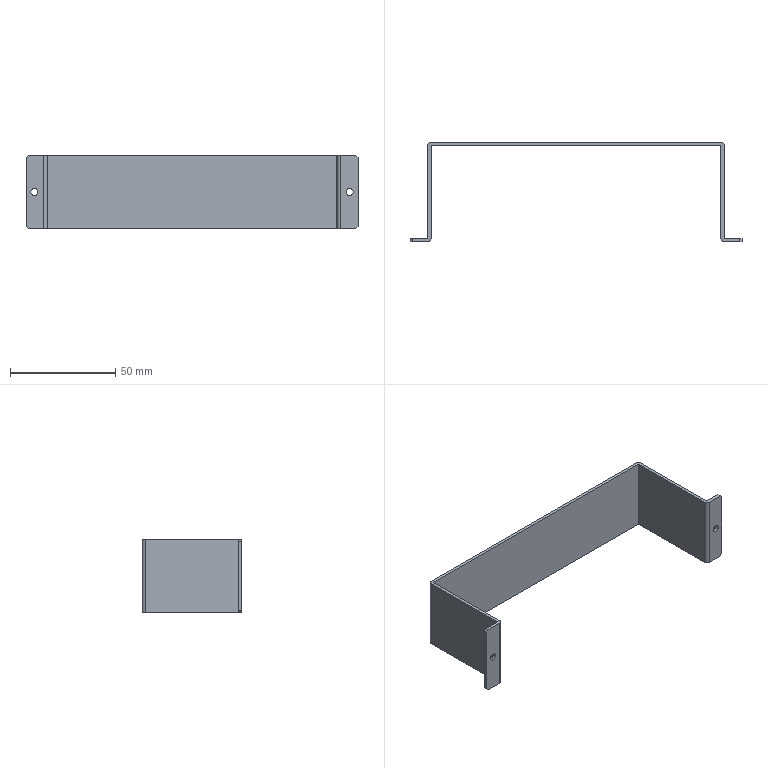Part | NX | 1 solid | 24 faces | box 158 x 47.5 x 35 mm | volume 13029 mm3 | plane 18 | cylinder 6 | commonest cylinder face diameters 3 x4 3.3 x2
STEP:
#1=CARTESIAN_POINT('',(-70.5,-1.5,35.));
#2=VERTEX_POINT('',#1);
#3=CARTESIAN_POINT('',(-70.5,-46.,35.));
#4=VERTEX_POINT('',#3);
#5=CARTESIAN_POINT('',(-70.5,0.,35.));
#6=DIRECTION('',(0.,-1.,0.));
#7=VECTOR('',#6,1000.);
#8=LINE('',#5,#7);
#9=EDGE_CURVE('',#2,#4,#8,.T.);
#10=ORIENTED_EDGE('',*,*,#9,.F.);
#11=CARTESIAN_POINT('',(-70.5,-1.5,0.));
#12=VERTEX_POINT('',#11);
#13=CARTESIAN_POINT('',(-70.5,-1.5,35.));
#14=DIRECTION('',(0.,0.,-1.));
#15=VECTOR('',#14,1000.);
#16=LINE('',#13,#15);
#17=EDGE_CURVE('',#2,#12,#16,.T.);
#18=ORIENTED_EDGE('',*,*,#17,.T.);
#19=CARTESIAN_POINT('',(-70.5,-46.,0.));
#20=VERTEX_POINT('',#19);
#21=CARTESIAN_POINT('',(-70.5,0.,0.));
#22=DIRECTION('',(0.,-1.,0.));
#23=VECTOR('',#22,1000.);
#24=LINE('',#21,#23);
#25=EDGE_CURVE('',#12,#20,#24,.T.);
#26=ORIENTED_EDGE('',*,*,#25,.T.);
#27=CARTESIAN_POINT('',(-70.5,-46.,35.));
#28=DIRECTION('',(0.,0.,-1.));
#29=VECTOR('',#28,1000.);
#30=LINE('',#27,#29);
#31=EDGE_CURVE('',#4,#20,#30,.T.);
#32=ORIENTED_EDGE('',*,*,#31,.F.);
#33=EDGE_LOOP('',(#10,#18,#26,#32));
#34=FACE_BOUND('',#33,.T.);
#35=CARTESIAN_POINT('',(-70.5,0.,35.));
#36=DIRECTION('',(1.,0.,0.));
#37=DIRECTION('',(0.,0.,-1.));
#38=AXIS2_PLACEMENT_3D('',#35,#36,#37);
#39=PLANE('',#38);
#40=ADVANCED_FACE('',(#34),#39,.F.);
#41=CARTESIAN_POINT('',(-75.,-46.,19.15));
#42=VERTEX_POINT('',#41);
#43=CARTESIAN_POINT('',(-75.,-46.,17.5));
#44=DIRECTION('',(0.,1.,0.));
#45=DIRECTION('',(0.,0.,1.));
#46=AXIS2_PLACEMENT_3D('',#43,#44,#45);
#47=CIRCLE('',#46,1.65);
#48=EDGE_CURVE('',#42,#42,#47,.T.);
#49=ORIENTED_EDGE('',*,*,#48,.F.);
#50=EDGE_LOOP('',(#49));
#51=FACE_BOUND('',#50,.T.);
#52=CARTESIAN_POINT('',(-78.,-46.,0.));
#53=VERTEX_POINT('',#52);
#54=CARTESIAN_POINT('',(-70.5,-46.,0.));
#55=DIRECTION('',(-1.,0.,0.));
#56=VECTOR('',#55,1000.);
#57=LINE('',#54,#56);
#58=EDGE_CURVE('',#20,#53,#57,.T.);
#59=ORIENTED_EDGE('',*,*,#58,.T.);
#60=CARTESIAN_POINT('',(-79.,-46.,1.));
#61=VERTEX_POINT('',#60);
#62=CARTESIAN_POINT('',(-79.,-46.,1.));
#63=DIRECTION('',(-0.7071,0.,0.7071));
#64=VECTOR('',#63,1000.);
#65=LINE('',#62,#64);
#66=EDGE_CURVE('',#53,#61,#65,.T.);
#67=ORIENTED_EDGE('',*,*,#66,.T.);
#68=CARTESIAN_POINT('',(-79.,-46.,34.));
#69=VERTEX_POINT('',#68);
#70=CARTESIAN_POINT('',(-79.,-46.,35.));
#71=DIRECTION('',(0.,0.,-1.));
#72=VECTOR('',#71,1000.);
#73=LINE('',#70,#72);
#74=EDGE_CURVE('',#69,#61,#73,.T.);
#75=ORIENTED_EDGE('',*,*,#74,.F.);
#76=CARTESIAN_POINT('',(-78.,-46.,35.));
#77=VERTEX_POINT('',#76);
#78=CARTESIAN_POINT('',(-78.,-46.,35.));
#79=DIRECTION('',(-0.7071,0.,-0.7071));
#80=VECTOR('',#79,1000.);
#81=LINE('',#78,#80);
#82=EDGE_CURVE('',#69,#77,#81,.F.);
#83=ORIENTED_EDGE('',*,*,#82,.T.);
#84=CARTESIAN_POINT('',(-70.5,-46.,35.));
#85=DIRECTION('',(-1.,0.,0.));
#86=VECTOR('',#85,1000.);
#87=LINE('',#84,#86);
#88=EDGE_CURVE('',#4,#77,#87,.T.);
#89=ORIENTED_EDGE('',*,*,#88,.F.);
#90=ORIENTED_EDGE('',*,*,#31,.T.);
#91=EDGE_LOOP('',(#59,#67,#75,#83,#89,#90));
#92=FACE_BOUND('',#91,.T.);
#93=CARTESIAN_POINT('',(-70.5,-46.,35.));
#94=DIRECTION('',(0.,-1.,0.));
#95=DIRECTION('',(0.,0.,-1.));
#96=AXIS2_PLACEMENT_3D('',#93,#94,#95);
#97=PLANE('',#96);
#98=ADVANCED_FACE('',(#51,#92),#97,.F.);
#99=ORIENTED_EDGE('',*,*,#74,.T.);
#100=CARTESIAN_POINT('',(-79.,-47.5,1.));
#101=VERTEX_POINT('',#100);
#102=CARTESIAN_POINT('',(-79.,-47.5,1.));
#103=DIRECTION('',(0.,-1.,0.));
#104=VECTOR('',#103,1000.);
#105=LINE('',#102,#104);
#106=EDGE_CURVE('',#61,#101,#105,.T.);
#107=ORIENTED_EDGE('',*,*,#106,.T.);
#108=CARTESIAN_POINT('',(-79.,-47.5,34.));
#109=VERTEX_POINT('',#108);
#110=CARTESIAN_POINT('',(-79.,-47.5,35.));
#111=DIRECTION('',(0.,0.,-1.));
#112=VECTOR('',#111,1000.);
#113=LINE('',#110,#112);
#114=EDGE_CURVE('',#109,#101,#113,.T.);
#115=ORIENTED_EDGE('',*,*,#114,.F.);
#116=CARTESIAN_POINT('',(-79.,-46.,34.));
#117=DIRECTION('',(0.,1.,0.));
#118=VECTOR('',#117,1000.);
#119=LINE('',#116,#118);
#120=EDGE_CURVE('',#109,#69,#119,.T.);
#121=ORIENTED_EDGE('',*,*,#120,.T.);
#122=EDGE_LOOP('',(#99,#107,#115,#121));
#123=FACE_BOUND('',#122,.T.);
#124=CARTESIAN_POINT('',(-79.,-46.,35.));
#125=DIRECTION('',(1.,0.,0.));
#126=DIRECTION('',(0.,0.,-1.));
#127=AXIS2_PLACEMENT_3D('',#124,#125,#126);
#128=PLANE('',#127);
#129=ADVANCED_FACE('',(#123),#128,.F.);
#130=CARTESIAN_POINT('',(-75.,-47.5,19.15));
#131=VERTEX_POINT('',#130);
#132=CARTESIAN_POINT('',(-75.,-47.5,17.5));
#133=DIRECTION('',(0.,1.,0.));
#134=DIRECTION('',(0.,0.,1.));
#135=AXIS2_PLACEMENT_3D('',#132,#133,#134);
#136=CIRCLE('',#135,1.65);
#137=EDGE_CURVE('',#131,#131,#136,.T.);
#138=ORIENTED_EDGE('',*,*,#137,.T.);
#139=EDGE_LOOP('',(#138));
#140=FACE_BOUND('',#139,.T.);
#141=ORIENTED_EDGE('',*,*,#114,.T.);
#142=CARTESIAN_POINT('',(-78.,-47.5,0.));
#143=VERTEX_POINT('',#142);
#144=CARTESIAN_POINT('',(-79.,-47.5,1.));
#145=DIRECTION('',(0.7071,0.,-0.7071));
#146=VECTOR('',#145,1000.);
#147=LINE('',#144,#146);
#148=EDGE_CURVE('',#101,#143,#147,.T.);
#149=ORIENTED_EDGE('',*,*,#148,.T.);
#150=CARTESIAN_POINT('',(-70.5,-47.5,0.));
#151=VERTEX_POINT('',#150);
#152=CARTESIAN_POINT('',(-79.,-47.5,0.));
#153=DIRECTION('',(1.,0.,0.));
#154=VECTOR('',#153,1000.);
#155=LINE('',#152,#154);
#156=EDGE_CURVE('',#143,#151,#155,.T.);
#157=ORIENTED_EDGE('',*,*,#156,.T.);
#158=CARTESIAN_POINT('',(-70.5,-47.5,35.));
#159=VERTEX_POINT('',#158);
#160=CARTESIAN_POINT('',(-70.5,-47.5,35.));
#161=DIRECTION('',(0.,0.,-1.));
#162=VECTOR('',#161,1000.);
#163=LINE('',#160,#162);
#164=EDGE_CURVE('',#151,#159,#163,.F.);
#165=ORIENTED_EDGE('',*,*,#164,.T.);
#166=CARTESIAN_POINT('',(-78.,-47.5,35.));
#167=VERTEX_POINT('',#166);
#168=CARTESIAN_POINT('',(-79.,-47.5,35.));
#169=DIRECTION('',(1.,0.,0.));
#170=VECTOR('',#169,1000.);
#171=LINE('',#168,#170);
#172=EDGE_CURVE('',#167,#159,#171,.T.);
#173=ORIENTED_EDGE('',*,*,#172,.F.);
#174=CARTESIAN_POINT('',(-78.,-47.5,35.));
#175=DIRECTION('',(0.7071,0.,0.7071));
#176=VECTOR('',#175,1000.);
#177=LINE('',#174,#176);
#178=EDGE_CURVE('',#167,#109,#177,.F.);
#179=ORIENTED_EDGE('',*,*,#178,.T.);
#180=EDGE_LOOP('',(#141,#149,#157,#165,#173,#179));
#181=FACE_BOUND('',#180,.T.);
#182=CARTESIAN_POINT('',(-79.,-47.5,35.));
#183=DIRECTION('',(0.,1.,0.));
#184=DIRECTION('',(0.,0.,1.));
#185=AXIS2_PLACEMENT_3D('',#182,#183,#184);
#186=PLANE('',#185);
#187=ADVANCED_FACE('',(#140,#181),#186,.F.);
#188=CARTESIAN_POINT('',(-69.,-46.,35.));
#189=VERTEX_POINT('',#188);
#190=CARTESIAN_POINT('',(-69.,-1.5,35.));
#191=VERTEX_POINT('',#190);
#192=CARTESIAN_POINT('',(-69.,-47.5,35.));
#193=DIRECTION('',(0.,1.,0.));
#194=VECTOR('',#193,1000.);
#195=LINE('',#192,#194);
#196=EDGE_CURVE('',#189,#191,#195,.T.);
#197=ORIENTED_EDGE('',*,*,#196,.F.);
#198=CARTESIAN_POINT('',(-69.,-46.,0.));
#199=VERTEX_POINT('',#198);
#200=CARTESIAN_POINT('',(-69.,-46.,35.));
#201=DIRECTION('',(0.,0.,-1.));
#202=VECTOR('',#201,1000.);
#203=LINE('',#200,#202);
#204=EDGE_CURVE('',#189,#199,#203,.T.);
#205=ORIENTED_EDGE('',*,*,#204,.T.);
#206=CARTESIAN_POINT('',(-69.,-1.5,0.));
#207=VERTEX_POINT('',#206);
#208=CARTESIAN_POINT('',(-69.,-47.5,0.));
#209=DIRECTION('',(0.,1.,0.));
#210=VECTOR('',#209,1000.);
#211=LINE('',#208,#210);
#212=EDGE_CURVE('',#199,#207,#211,.T.);
#213=ORIENTED_EDGE('',*,*,#212,.T.);
#214=CARTESIAN_POINT('',(-69.,-1.5,35.));
#215=DIRECTION('',(0.,0.,-1.));
#216=VECTOR('',#215,1000.);
#217=LINE('',#214,#216);
#218=EDGE_CURVE('',#191,#207,#217,.T.);
#219=ORIENTED_EDGE('',*,*,#218,.F.);
#220=EDGE_LOOP('',(#197,#205,#213,#219));
#221=FACE_BOUND('',#220,.T.);
#222=CARTESIAN_POINT('',(-69.,-47.5,35.));
#223=DIRECTION('',(-1.,0.,0.));
#224=DIRECTION('',(0.,0.,1.));
#225=AXIS2_PLACEMENT_3D('',#222,#223,#224);
#226=PLANE('',#225);
#227=ADVANCED_FACE('',(#221),#226,.F.);
#228=CARTESIAN_POINT('',(69.,-1.5,0.));
#229=VERTEX_POINT('',#228);
#230=CARTESIAN_POINT('',(69.,-1.5,0.));
#231=DIRECTION('',(1.,0.,0.));
#232=VECTOR('',#231,1000.);
#233=LINE('',#230,#232);
#234=EDGE_CURVE('',#207,#229,#233,.T.);
#235=ORIENTED_EDGE('',*,*,#234,.T.);
#236=CARTESIAN_POINT('',(69.,-1.5,35.));
#237=VERTEX_POINT('',#236);
#238=CARTESIAN_POINT('',(69.,-1.5,35.));
#239=DIRECTION('',(0.,0.,-1.));
#240=VECTOR('',#239,1000.);
#241=LINE('',#238,#240);
#242=EDGE_CURVE('',#237,#229,#241,.T.);
#243=ORIENTED_EDGE('',*,*,#242,.F.);
#244=CARTESIAN_POINT('',(69.,-1.5,35.));
#245=DIRECTION('',(1.,0.,0.));
#246=VECTOR('',#245,1000.);
#247=LINE('',#244,#246);
#248=EDGE_CURVE('',#191,#237,#247,.T.);
#249=ORIENTED_EDGE('',*,*,#248,.F.);
#250=ORIENTED_EDGE('',*,*,#218,.T.);
#251=EDGE_LOOP('',(#235,#243,#249,#250));
#252=FACE_BOUND('',#251,.T.);
#253=CARTESIAN_POINT('',(69.,-1.5,35.));
#254=DIRECTION('',(0.,1.,0.));
#255=DIRECTION('',(-1.,0.,0.));
#256=AXIS2_PLACEMENT_3D('',#253,#254,#255);
#257=PLANE('',#256);
#258=ADVANCED_FACE('',(#252),#257,.F.);
#259=CARTESIAN_POINT('',(69.,-46.,0.));
#260=VERTEX_POINT('',#259);
#261=CARTESIAN_POINT('',(69.,-47.5,0.));
#262=DIRECTION('',(0.,-1.,0.));
#263=VECTOR('',#262,1000.);
#264=LINE('',#261,#263);
#265=EDGE_CURVE('',#229,#260,#264,.T.);
#266=ORIENTED_EDGE('',*,*,#265,.T.);
#267=CARTESIAN_POINT('',(69.,-46.,35.));
#268=VERTEX_POINT('',#267);
#269=CARTESIAN_POINT('',(69.,-46.,35.));
#270=DIRECTION('',(0.,0.,-1.));
#271=VECTOR('',#270,1000.);
#272=LINE('',#269,#271);
#273=EDGE_CURVE('',#260,#268,#272,.F.);
#274=ORIENTED_EDGE('',*,*,#273,.T.);
#275=CARTESIAN_POINT('',(69.,-47.5,35.));
#276=DIRECTION('',(0.,-1.,0.));
#277=VECTOR('',#276,1000.);
#278=LINE('',#275,#277);
#279=EDGE_CURVE('',#237,#268,#278,.T.);
#280=ORIENTED_EDGE('',*,*,#279,.F.);
#281=ORIENTED_EDGE('',*,*,#242,.T.);
#282=EDGE_LOOP('',(#266,#274,#280,#281));
#283=FACE_BOUND('',#282,.T.);
#284=CARTESIAN_POINT('',(69.,-47.5,35.));
#285=DIRECTION('',(1.,0.,0.));
#286=DIRECTION('',(0.,0.,-1.));
#287=AXIS2_PLACEMENT_3D('',#284,#285,#286);
#288=PLANE('',#287);
#289=ADVANCED_FACE('',(#283),#288,.F.);
#290=CARTESIAN_POINT('',(75.,-47.5,19.15));
#291=VERTEX_POINT('',#290);
#292=CARTESIAN_POINT('',(75.,-47.5,17.5));
#293=DIRECTION('',(0.,1.,0.));
#294=DIRECTION('',(0.,0.,1.));
#295=AXIS2_PLACEMENT_3D('',#292,#293,#294);
#296=CIRCLE('',#295,1.65);
#297=EDGE_CURVE('',#291,#291,#296,.T.);
#298=ORIENTED_EDGE('',*,*,#297,.T.);
#299=EDGE_LOOP('',(#298));
#300=FACE_BOUND('',#299,.T.);
#301=CARTESIAN_POINT('',(70.5,-47.5,0.));
#302=VERTEX_POINT('',#301);
#303=CARTESIAN_POINT('',(78.,-47.5,0.));
#304=VERTEX_POINT('',#303);
#305=CARTESIAN_POINT('',(79.,-47.5,0.));
#306=DIRECTION('',(1.,0.,0.));
#307=VECTOR('',#306,1000.);
#308=LINE('',#305,#307);
#309=EDGE_CURVE('',#302,#304,#308,.T.);
#310=ORIENTED_EDGE('',*,*,#309,.T.);
#311=CARTESIAN_POINT('',(79.,-47.5,1.));
#312=VERTEX_POINT('',#311);
#313=CARTESIAN_POINT('',(79.,-47.5,1.));
#314=DIRECTION('',(0.7071,0.,0.7071));
#315=VECTOR('',#314,1000.);
#316=LINE('',#313,#315);
#317=EDGE_CURVE('',#304,#312,#316,.T.);
#318=ORIENTED_EDGE('',*,*,#317,.T.);
#319=CARTESIAN_POINT('',(79.,-47.5,34.));
#320=VERTEX_POINT('',#319);
#321=CARTESIAN_POINT('',(79.,-47.5,35.));
#322=DIRECTION('',(0.,0.,-1.));
#323=VECTOR('',#322,1000.);
#324=LINE('',#321,#323);
#325=EDGE_CURVE('',#320,#312,#324,.T.);
#326=ORIENTED_EDGE('',*,*,#325,.F.);
#327=CARTESIAN_POINT('',(78.,-47.5,35.));
#328=VERTEX_POINT('',#327);
#329=CARTESIAN_POINT('',(78.,-47.5,35.));
#330=DIRECTION('',(0.7071,0.,-0.7071));
#331=VECTOR('',#330,1000.);
#332=LINE('',#329,#331);
#333=EDGE_CURVE('',#320,#328,#332,.F.);
#334=ORIENTED_EDGE('',*,*,#333,.T.);
#335=CARTESIAN_POINT('',(70.5,-47.5,35.));
#336=VERTEX_POINT('',#335);
#337=CARTESIAN_POINT('',(79.,-47.5,35.));
#338=DIRECTION('',(1.,0.,0.));
#339=VECTOR('',#338,1000.);
#340=LINE('',#337,#339);
#341=EDGE_CURVE('',#336,#328,#340,.T.);
#342=ORIENTED_EDGE('',*,*,#341,.F.);
#343=CARTESIAN_POINT('',(70.5,-47.5,35.));
#344=DIRECTION('',(0.,0.,-1.));
#345=VECTOR('',#344,1000.);
#346=LINE('',#343,#345);
#347=EDGE_CURVE('',#336,#302,#346,.T.);
#348=ORIENTED_EDGE('',*,*,#347,.T.);
#349=EDGE_LOOP('',(#310,#318,#326,#334,#342,#348));
#350=FACE_BOUND('',#349,.T.);
#351=CARTESIAN_POINT('',(79.,-47.5,35.));
#352=DIRECTION('',(0.,1.,0.));
#353=DIRECTION('',(0.,0.,1.));
#354=AXIS2_PLACEMENT_3D('',#351,#352,#353);
#355=PLANE('',#354);
#356=ADVANCED_FACE('',(#300,#350),#355,.F.);
#357=ORIENTED_EDGE('',*,*,#325,.T.);
#358=CARTESIAN_POINT('',(79.,-46.,1.));
#359=VERTEX_POINT('',#358);
#360=CARTESIAN_POINT('',(79.,-46.,1.));
#361=DIRECTION('',(0.,1.,0.));
#362=VECTOR('',#361,1000.);
#363=LINE('',#360,#362);
#364=EDGE_CURVE('',#312,#359,#363,.T.);
#365=ORIENTED_EDGE('',*,*,#364,.T.);
#366=CARTESIAN_POINT('',(79.,-46.,34.));
#367=VERTEX_POINT('',#366);
#368=CARTESIAN_POINT('',(79.,-46.,35.));
#369=DIRECTION('',(0.,0.,-1.));
#370=VECTOR('',#369,1000.);
#371=LINE('',#368,#370);
#372=EDGE_CURVE('',#367,#359,#371,.T.);
#373=ORIENTED_EDGE('',*,*,#372,.F.);
#374=CARTESIAN_POINT('',(79.,-46.,34.));
#375=DIRECTION('',(0.,-1.,0.));
#376=VECTOR('',#375,1000.);
#377=LINE('',#374,#376);
#378=EDGE_CURVE('',#367,#320,#377,.T.);
#379=ORIENTED_EDGE('',*,*,#378,.T.);
#380=EDGE_LOOP('',(#357,#365,#373,#379));
#381=FACE_BOUND('',#380,.T.);
#382=CARTESIAN_POINT('',(79.,-46.,35.));
#383=DIRECTION('',(-1.,0.,0.));
#384=DIRECTION('',(0.,0.,1.));
#385=AXIS2_PLACEMENT_3D('',#382,#383,#384);
#386=PLANE('',#385);
#387=ADVANCED_FACE('',(#381),#386,.F.);
#388=CARTESIAN_POINT('',(75.,-46.,19.15));
#389=VERTEX_POINT('',#388);
#390=CARTESIAN_POINT('',(75.,-46.,17.5));
#391=DIRECTION('',(0.,1.,0.));
#392=DIRECTION('',(0.,0.,1.));
#393=AXIS2_PLACEMENT_3D('',#390,#391,#392);
#394=CIRCLE('',#393,1.65);
#395=EDGE_CURVE('',#389,#389,#394,.T.);
#396=ORIENTED_EDGE('',*,*,#395,.F.);
#397=EDGE_LOOP('',(#396));
#398=FACE_BOUND('',#397,.T.);
#399=ORIENTED_EDGE('',*,*,#372,.T.);
#400=CARTESIAN_POINT('',(78.,-46.,0.));
#401=VERTEX_POINT('',#400);
#402=CARTESIAN_POINT('',(79.,-46.,1.));
#403=DIRECTION('',(-0.7071,0.,-0.7071));
#404=VECTOR('',#403,1000.);
#405=LINE('',#402,#404);
#406=EDGE_CURVE('',#359,#401,#405,.T.);
#407=ORIENTED_EDGE('',*,*,#406,.T.);
#408=CARTESIAN_POINT('',(70.5,-46.,0.));
#409=VERTEX_POINT('',#408);
#410=CARTESIAN_POINT('',(70.5,-46.,0.));
#411=DIRECTION('',(-1.,0.,0.));
#412=VECTOR('',#411,1000.);
#413=LINE('',#410,#412);
#414=EDGE_CURVE('',#401,#409,#413,.T.);
#415=ORIENTED_EDGE('',*,*,#414,.T.);
#416=CARTESIAN_POINT('',(70.5,-46.,35.));
#417=VERTEX_POINT('',#416);
#418=CARTESIAN_POINT('',(70.5,-46.,35.));
#419=DIRECTION('',(0.,0.,-1.));
#420=VECTOR('',#419,1000.);
#421=LINE('',#418,#420);
#422=EDGE_CURVE('',#417,#409,#421,.T.);
#423=ORIENTED_EDGE('',*,*,#422,.F.);
#424=CARTESIAN_POINT('',(78.,-46.,35.));
#425=VERTEX_POINT('',#424);
#426=CARTESIAN_POINT('',(70.5,-46.,35.));
#427=DIRECTION('',(-1.,0.,0.));
#428=VECTOR('',#427,1000.);
#429=LINE('',#426,#428);
#430=EDGE_CURVE('',#425,#417,#429,.T.);
#431=ORIENTED_EDGE('',*,*,#430,.F.);
#432=CARTESIAN_POINT('',(78.,-46.,35.));
#433=DIRECTION('',(-0.7071,0.,0.7071));
#434=VECTOR('',#433,1000.);
#435=LINE('',#432,#434);
#436=EDGE_CURVE('',#425,#367,#435,.F.);
#437=ORIENTED_EDGE('',*,*,#436,.T.);
#438=EDGE_LOOP('',(#399,#407,#415,#423,#431,#437));
#439=FACE_BOUND('',#438,.T.);
#440=CARTESIAN_POINT('',(70.5,-46.,35.));
#441=DIRECTION('',(0.,-1.,0.));
#442=DIRECTION('',(0.,0.,-1.));
#443=AXIS2_PLACEMENT_3D('',#440,#441,#442);
#444=PLANE('',#443);
#445=ADVANCED_FACE('',(#398,#439),#444,.F.);
#446=CARTESIAN_POINT('',(70.5,-1.5,0.));
#447=VERTEX_POINT('',#446);
#448=CARTESIAN_POINT('',(70.5,0.,0.));
#449=DIRECTION('',(0.,1.,0.));
#450=VECTOR('',#449,1000.);
#451=LINE('',#448,#450);
#452=EDGE_CURVE('',#409,#447,#451,.T.);
#453=ORIENTED_EDGE('',*,*,#452,.T.);
#454=CARTESIAN_POINT('',(70.5,-1.5,35.));
#455=VERTEX_POINT('',#454);
#456=CARTESIAN_POINT('',(70.5,-1.5,35.));
#457=DIRECTION('',(0.,0.,-1.));
#458=VECTOR('',#457,1000.);
#459=LINE('',#456,#458);
#460=EDGE_CURVE('',#447,#455,#459,.F.);
#461=ORIENTED_EDGE('',*,*,#460,.T.);
#462=CARTESIAN_POINT('',(70.5,0.,35.));
#463=DIRECTION('',(0.,1.,0.));
#464=VECTOR('',#463,1000.);
#465=LINE('',#462,#464);
#466=EDGE_CURVE('',#417,#455,#465,.T.);
#467=ORIENTED_EDGE('',*,*,#466,.F.);
#468=ORIENTED_EDGE('',*,*,#422,.T.);
#469=EDGE_LOOP('',(#453,#461,#467,#468));
#470=FACE_BOUND('',#469,.T.);
#471=CARTESIAN_POINT('',(70.5,0.,35.));
#472=DIRECTION('',(-1.,0.,0.));
#473=DIRECTION('',(0.,0.,1.));
#474=AXIS2_PLACEMENT_3D('',#471,#472,#473);
#475=PLANE('',#474);
#476=ADVANCED_FACE('',(#470),#475,.F.);
#477=CARTESIAN_POINT('',(69.,0.,35.));
#478=VERTEX_POINT('',#477);
#479=CARTESIAN_POINT('',(-69.,0.,35.));
#480=VERTEX_POINT('',#479);
#481=CARTESIAN_POINT('',(-70.5,0.,35.));
#482=DIRECTION('',(-1.,0.,0.));
#483=VECTOR('',#482,1000.);
#484=LINE('',#481,#483);
#485=EDGE_CURVE('',#478,#480,#484,.T.);
#486=ORIENTED_EDGE('',*,*,#485,.F.);
#487=CARTESIAN_POINT('',(69.,0.,0.));
#488=VERTEX_POINT('',#487);
#489=CARTESIAN_POINT('',(69.,0.,35.));
#490=DIRECTION('',(0.,0.,-1.));
#491=VECTOR('',#490,1000.);
#492=LINE('',#489,#491);
#493=EDGE_CURVE('',#478,#488,#492,.T.);
#494=ORIENTED_EDGE('',*,*,#493,.T.);
#495=CARTESIAN_POINT('',(-69.,0.,0.));
#496=VERTEX_POINT('',#495);
#497=CARTESIAN_POINT('',(-70.5,0.,0.));
#498=DIRECTION('',(-1.,0.,0.));
#499=VECTOR('',#498,1000.);
#500=LINE('',#497,#499);
#501=EDGE_CURVE('',#488,#496,#500,.T.);
#502=ORIENTED_EDGE('',*,*,#501,.T.);
#503=CARTESIAN_POINT('',(-69.,0.,35.));
#504=DIRECTION('',(0.,0.,-1.));
#505=VECTOR('',#504,1000.);
#506=LINE('',#503,#505);
#507=EDGE_CURVE('',#496,#480,#506,.F.);
#508=ORIENTED_EDGE('',*,*,#507,.T.);
#509=EDGE_LOOP('',(#486,#494,#502,#508));
#510=FACE_BOUND('',#509,.T.);
#511=CARTESIAN_POINT('',(-70.5,0.,35.));
#512=DIRECTION('',(0.,-1.,0.));
#513=DIRECTION('',(0.,0.,-1.));
#514=AXIS2_PLACEMENT_3D('',#511,#512,#513);
#515=PLANE('',#514);
#516=ADVANCED_FACE('',(#510),#515,.F.);
#517=ORIENTED_EDGE('',*,*,#341,.T.);
#518=CARTESIAN_POINT('',(78.,0.,35.));
#519=DIRECTION('',(0.,1.,0.));
#520=VECTOR('',#519,1000.);
#521=LINE('',#518,#520);
#522=EDGE_CURVE('',#328,#425,#521,.T.);
#523=ORIENTED_EDGE('',*,*,#522,.T.);
#524=ORIENTED_EDGE('',*,*,#430,.T.);
#525=ORIENTED_EDGE('',*,*,#466,.T.);
#526=CARTESIAN_POINT('',(69.,-1.5,35.));
#527=DIRECTION('',(0.,0.,-1.));
#528=DIRECTION('',(-1.,0.,0.));
#529=AXIS2_PLACEMENT_3D('',#526,#527,#528);
#530=CIRCLE('',#529,1.5);
#531=EDGE_CURVE('',#455,#478,#530,.F.);
#532=ORIENTED_EDGE('',*,*,#531,.T.);
#533=ORIENTED_EDGE('',*,*,#485,.T.);
#534=CARTESIAN_POINT('',(-69.,-1.5,35.));
#535=DIRECTION('',(0.,0.,-1.));
#536=DIRECTION('',(-1.,0.,0.));
#537=AXIS2_PLACEMENT_3D('',#534,#535,#536);
#538=CIRCLE('',#537,1.5);
#539=EDGE_CURVE('',#480,#2,#538,.F.);
#540=ORIENTED_EDGE('',*,*,#539,.T.);
#541=ORIENTED_EDGE('',*,*,#9,.T.);
#542=ORIENTED_EDGE('',*,*,#88,.T.);
#543=CARTESIAN_POINT('',(-78.,0.,35.));
#544=DIRECTION('',(0.,-1.,0.));
#545=VECTOR('',#544,1000.);
#546=LINE('',#543,#545);
#547=EDGE_CURVE('',#77,#167,#546,.T.);
#548=ORIENTED_EDGE('',*,*,#547,.T.);
#549=ORIENTED_EDGE('',*,*,#172,.T.);
#550=CARTESIAN_POINT('',(-70.5,-46.,35.));
#551=DIRECTION('',(0.,0.,-1.));
#552=DIRECTION('',(-1.,0.,0.));
#553=AXIS2_PLACEMENT_3D('',#550,#551,#552);
#554=CIRCLE('',#553,1.5);
#555=EDGE_CURVE('',#159,#189,#554,.F.);
#556=ORIENTED_EDGE('',*,*,#555,.T.);
#557=ORIENTED_EDGE('',*,*,#196,.T.);
#558=ORIENTED_EDGE('',*,*,#248,.T.);
#559=ORIENTED_EDGE('',*,*,#279,.T.);
#560=CARTESIAN_POINT('',(70.5,-46.,35.));
#561=DIRECTION('',(0.,0.,-1.));
#562=DIRECTION('',(-1.,0.,0.));
#563=AXIS2_PLACEMENT_3D('',#560,#561,#562);
#564=CIRCLE('',#563,1.5);
#565=EDGE_CURVE('',#268,#336,#564,.F.);
#566=ORIENTED_EDGE('',*,*,#565,.T.);
#567=EDGE_LOOP('',(#517,#523,#524,#525,#532,#533,#540,#541,#542,#548,#549,#556,#557,#558,#559,#566));
#568=FACE_BOUND('',#567,.T.);
#569=CARTESIAN_POINT('',(0.,0.,35.));
#570=DIRECTION('',(0.,0.,-1.));
#571=DIRECTION('',(-1.,0.,0.));
#572=AXIS2_PLACEMENT_3D('',#569,#570,#571);
#573=PLANE('',#572);
#574=ADVANCED_FACE('',(#568),#573,.F.);
#575=ORIENTED_EDGE('',*,*,#414,.F.);
#576=CARTESIAN_POINT('',(78.,-47.5,0.));
#577=DIRECTION('',(0.,-1.,0.));
#578=VECTOR('',#577,1000.);
#579=LINE('',#576,#578);
#580=EDGE_CURVE('',#401,#304,#579,.T.);
#581=ORIENTED_EDGE('',*,*,#580,.T.);
#582=ORIENTED_EDGE('',*,*,#309,.F.);
#583=CARTESIAN_POINT('',(70.5,-46.,0.));
#584=DIRECTION('',(0.,0.,-1.));
#585=DIRECTION('',(-1.,0.,0.));
#586=AXIS2_PLACEMENT_3D('',#583,#584,#585);
#587=CIRCLE('',#586,1.5);
#588=EDGE_CURVE('',#302,#260,#587,.T.);
#589=ORIENTED_EDGE('',*,*,#588,.T.);
#590=ORIENTED_EDGE('',*,*,#265,.F.);
#591=ORIENTED_EDGE('',*,*,#234,.F.);
#592=ORIENTED_EDGE('',*,*,#212,.F.);
#593=CARTESIAN_POINT('',(-70.5,-46.,0.));
#594=DIRECTION('',(0.,0.,-1.));
#595=DIRECTION('',(-1.,0.,0.));
#596=AXIS2_PLACEMENT_3D('',#593,#594,#595);
#597=CIRCLE('',#596,1.5);
#598=EDGE_CURVE('',#199,#151,#597,.T.);
#599=ORIENTED_EDGE('',*,*,#598,.T.);
#600=ORIENTED_EDGE('',*,*,#156,.F.);
#601=CARTESIAN_POINT('',(-78.,-46.,0.));
#602=DIRECTION('',(0.,1.,0.));
#603=VECTOR('',#602,1000.);
#604=LINE('',#601,#603);
#605=EDGE_CURVE('',#143,#53,#604,.T.);
#606=ORIENTED_EDGE('',*,*,#605,.T.);
#607=ORIENTED_EDGE('',*,*,#58,.F.);
#608=ORIENTED_EDGE('',*,*,#25,.F.);
#609=CARTESIAN_POINT('',(-69.,-1.5,0.));
#610=DIRECTION('',(0.,0.,-1.));
#611=DIRECTION('',(-1.,0.,0.));
#612=AXIS2_PLACEMENT_3D('',#609,#610,#611);
#613=CIRCLE('',#612,1.5);
#614=EDGE_CURVE('',#12,#496,#613,.T.);
#615=ORIENTED_EDGE('',*,*,#614,.T.);
#616=ORIENTED_EDGE('',*,*,#501,.F.);
#617=CARTESIAN_POINT('',(69.,-1.5,0.));
#618=DIRECTION('',(0.,0.,-1.));
#619=DIRECTION('',(-1.,0.,0.));
#620=AXIS2_PLACEMENT_3D('',#617,#618,#619);
#621=CIRCLE('',#620,1.5);
#622=EDGE_CURVE('',#488,#447,#621,.T.);
#623=ORIENTED_EDGE('',*,*,#622,.T.);
#624=ORIENTED_EDGE('',*,*,#452,.F.);
#625=EDGE_LOOP('',(#575,#581,#582,#589,#590,#591,#592,#599,#600,#606,#607,#608,#615,#616,#623,#624));
#626=FACE_BOUND('',#625,.T.);
#627=CARTESIAN_POINT('',(0.,0.,0.));
#628=DIRECTION('',(0.,0.,-1.));
#629=DIRECTION('',(-1.,0.,0.));
#630=AXIS2_PLACEMENT_3D('',#627,#628,#629);
#631=PLANE('',#630);
#632=ADVANCED_FACE('',(#626),#631,.T.);
#633=ORIENTED_EDGE('',*,*,#531,.F.);
#634=ORIENTED_EDGE('',*,*,#460,.F.);
#635=ORIENTED_EDGE('',*,*,#622,.F.);
#636=ORIENTED_EDGE('',*,*,#493,.F.);
#637=EDGE_LOOP('',(#633,#634,#635,#636));
#638=FACE_BOUND('',#637,.T.);
#639=CARTESIAN_POINT('',(69.,-1.5,35.));
#640=DIRECTION('',(0.,0.,-1.));
#641=DIRECTION('',(-1.,0.,0.));
#642=AXIS2_PLACEMENT_3D('',#639,#640,#641);
#643=CYLINDRICAL_SURFACE('',#642,1.5);
#644=ADVANCED_FACE('',(#638),#643,.T.);
#645=ORIENTED_EDGE('',*,*,#565,.F.);
#646=ORIENTED_EDGE('',*,*,#273,.F.);
#647=ORIENTED_EDGE('',*,*,#588,.F.);
#648=ORIENTED_EDGE('',*,*,#347,.F.);
#649=EDGE_LOOP('',(#645,#646,#647,#648));
#650=FACE_BOUND('',#649,.T.);
#651=CARTESIAN_POINT('',(70.5,-46.,35.));
#652=DIRECTION('',(0.,0.,-1.));
#653=DIRECTION('',(-1.,0.,0.));
#654=AXIS2_PLACEMENT_3D('',#651,#652,#653);
#655=CYLINDRICAL_SURFACE('',#654,1.5);
#656=ADVANCED_FACE('',(#650),#655,.T.);
#657=ORIENTED_EDGE('',*,*,#555,.F.);
#658=ORIENTED_EDGE('',*,*,#164,.F.);
#659=ORIENTED_EDGE('',*,*,#598,.F.);
#660=ORIENTED_EDGE('',*,*,#204,.F.);
#661=EDGE_LOOP('',(#657,#658,#659,#660));
#662=FACE_BOUND('',#661,.T.);
#663=CARTESIAN_POINT('',(-70.5,-46.,35.));
#664=DIRECTION('',(0.,0.,-1.));
#665=DIRECTION('',(-1.,0.,0.));
#666=AXIS2_PLACEMENT_3D('',#663,#664,#665);
#667=CYLINDRICAL_SURFACE('',#666,1.5);
#668=ADVANCED_FACE('',(#662),#667,.T.);
#669=ORIENTED_EDGE('',*,*,#539,.F.);
#670=ORIENTED_EDGE('',*,*,#507,.F.);
#671=ORIENTED_EDGE('',*,*,#614,.F.);
#672=ORIENTED_EDGE('',*,*,#17,.F.);
#673=EDGE_LOOP('',(#669,#670,#671,#672));
#674=FACE_BOUND('',#673,.T.);
#675=CARTESIAN_POINT('',(-69.,-1.5,35.));
#676=DIRECTION('',(0.,0.,-1.));
#677=DIRECTION('',(-1.,0.,0.));
#678=AXIS2_PLACEMENT_3D('',#675,#676,#677);
#679=CYLINDRICAL_SURFACE('',#678,1.5);
#680=ADVANCED_FACE('',(#674),#679,.T.);
#681=ORIENTED_EDGE('',*,*,#48,.T.);
#682=EDGE_LOOP('',(#681));
#683=FACE_BOUND('',#682,.T.);
#684=ORIENTED_EDGE('',*,*,#137,.F.);
#685=EDGE_LOOP('',(#684));
#686=FACE_BOUND('',#685,.T.);
#687=CARTESIAN_POINT('',(-75.,-46.,17.5));
#688=DIRECTION('',(0.,1.,0.));
#689=DIRECTION('',(0.,0.,1.));
#690=AXIS2_PLACEMENT_3D('',#687,#688,#689);
#691=CYLINDRICAL_SURFACE('',#690,1.65);
#692=ADVANCED_FACE('',(#683,#686),#691,.F.);
#693=ORIENTED_EDGE('',*,*,#395,.T.);
#694=EDGE_LOOP('',(#693));
#695=FACE_BOUND('',#694,.T.);
#696=ORIENTED_EDGE('',*,*,#297,.F.);
#697=EDGE_LOOP('',(#696));
#698=FACE_BOUND('',#697,.T.);
#699=CARTESIAN_POINT('',(75.,-46.,17.5));
#700=DIRECTION('',(0.,1.,0.));
#701=DIRECTION('',(0.,0.,1.));
#702=AXIS2_PLACEMENT_3D('',#699,#700,#701);
#703=CYLINDRICAL_SURFACE('',#702,1.65);
#704=ADVANCED_FACE('',(#695,#698),#703,.F.);
#705=ORIENTED_EDGE('',*,*,#317,.F.);
#706=ORIENTED_EDGE('',*,*,#580,.F.);
#707=ORIENTED_EDGE('',*,*,#406,.F.);
#708=ORIENTED_EDGE('',*,*,#364,.F.);
#709=EDGE_LOOP('',(#705,#706,#707,#708));
#710=FACE_BOUND('',#709,.T.);
#711=CARTESIAN_POINT('',(79.,-46.,1.));
#712=DIRECTION('',(0.7071,0.,-0.7071));
#713=DIRECTION('',(0.,-1.,0.));
#714=AXIS2_PLACEMENT_3D('',#711,#712,#713);
#715=PLANE('',#714);
#716=ADVANCED_FACE('',(#710),#715,.T.);
#717=ORIENTED_EDGE('',*,*,#333,.F.);
#718=ORIENTED_EDGE('',*,*,#378,.F.);
#719=ORIENTED_EDGE('',*,*,#436,.F.);
#720=ORIENTED_EDGE('',*,*,#522,.F.);
#721=EDGE_LOOP('',(#717,#718,#719,#720));
#722=FACE_BOUND('',#721,.T.);
#723=CARTESIAN_POINT('',(78.,0.,35.));
#724=DIRECTION('',(-0.7071,0.,-0.7071));
#725=DIRECTION('',(0.,1.,0.));
#726=AXIS2_PLACEMENT_3D('',#723,#724,#725);
#727=PLANE('',#726);
#728=ADVANCED_FACE('',(#722),#727,.F.);
#729=ORIENTED_EDGE('',*,*,#66,.F.);
#730=ORIENTED_EDGE('',*,*,#605,.F.);
#731=ORIENTED_EDGE('',*,*,#148,.F.);
#732=ORIENTED_EDGE('',*,*,#106,.F.);
#733=EDGE_LOOP('',(#729,#730,#731,#732));
#734=FACE_BOUND('',#733,.T.);
#735=CARTESIAN_POINT('',(-79.,-46.,1.));
#736=DIRECTION('',(-0.7071,0.,-0.7071));
#737=DIRECTION('',(0.,1.,0.));
#738=AXIS2_PLACEMENT_3D('',#735,#736,#737);
#739=PLANE('',#738);
#740=ADVANCED_FACE('',(#734),#739,.T.);
#741=ORIENTED_EDGE('',*,*,#82,.F.);
#742=ORIENTED_EDGE('',*,*,#120,.F.);
#743=ORIENTED_EDGE('',*,*,#178,.F.);
#744=ORIENTED_EDGE('',*,*,#547,.F.);
#745=EDGE_LOOP('',(#741,#742,#743,#744));
#746=FACE_BOUND('',#745,.T.);
#747=CARTESIAN_POINT('',(-78.,0.,35.));
#748=DIRECTION('',(0.7071,0.,-0.7071));
#749=DIRECTION('',(0.,-1.,0.));
#750=AXIS2_PLACEMENT_3D('',#747,#748,#749);
#751=PLANE('',#750);
#752=ADVANCED_FACE('',(#746),#751,.F.);
#753=CLOSED_SHELL('',(#40,#98,#129,#187,#227,#258,#289,#356,#387,#445,#476,#516,#574,#632,#644,#656,#668,#680,#692,#704,#716,#728,#740,#752));
#754=MANIFOLD_SOLID_BREP('',#753);
#755=(LENGTH_UNIT()NAMED_UNIT(*)SI_UNIT(.MILLI.,.METRE.));
#756=UNCERTAINTY_MEASURE_WITH_UNIT(LENGTH_MEASURE(0.00001),#755,'','');
#757=(NAMED_UNIT(*)PLANE_ANGLE_UNIT()SI_UNIT($,.RADIAN.));
#758=(NAMED_UNIT(*)SI_UNIT($,.STERADIAN.)SOLID_ANGLE_UNIT());
#759=(GEOMETRIC_REPRESENTATION_CONTEXT(3)GLOBAL_UNCERTAINTY_ASSIGNED_CONTEXT((#756))GLOBAL_UNIT_ASSIGNED_CONTEXT((#755,#757,#758))REPRESENTATION_CONTEXT('',''));
#760=ADVANCED_BREP_SHAPE_REPRESENTATION('',(#754),#759);